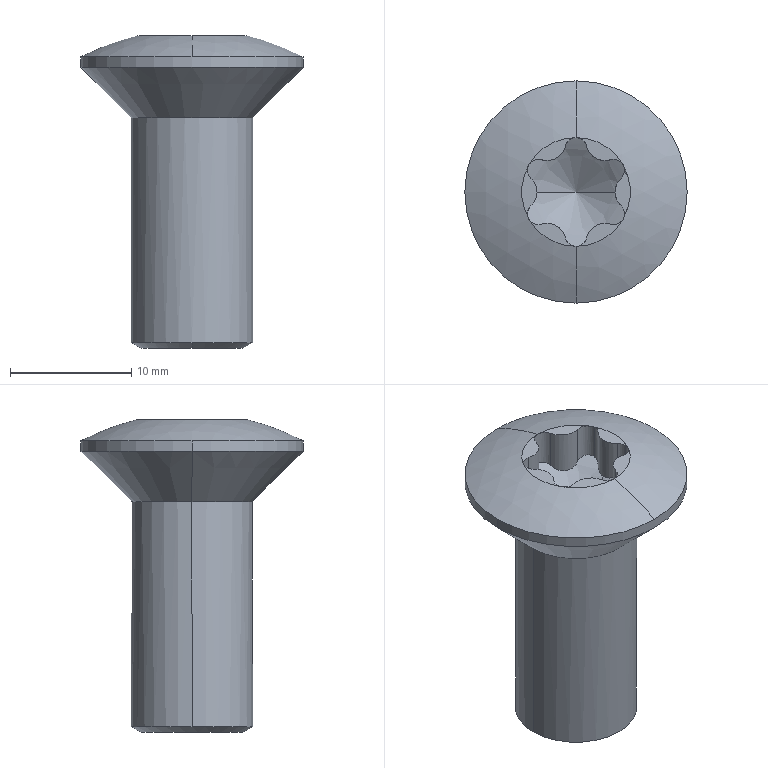Part | SolidWorks | features RevCut 2, ICE 1, LPattern 1, Revolution 1 | 1 solid | 34 faces | box 18.3 x 18.3 x 25.76 mm | volume 2486 mm3 | cylinder 19 | plane 7 | cone 6 | sphere 2 | commonest cylinder face diameters 1.79 x8 3.132 x7 10 x2 18.3 x2
STEP:
#1=CARTESIAN_POINT('',(0.,4.172,-26.28));
#2=VERTEX_POINT('',#1);
#3=CARTESIAN_POINT('',(0.,-4.172,-26.28));
#4=VERTEX_POINT('',#3);
#5=CARTESIAN_POINT('',(0.,0.,-26.28));
#6=DIRECTION('',(0.,0.,-1.));
#7=DIRECTION('',(0.,1.,0.));
#8=AXIS2_PLACEMENT_3D('',#5,#6,#7);
#9=CIRCLE('',#8,4.172);
#10=EDGE_CURVE('',#2,#4,#9,.T.);
#11=ORIENTED_EDGE('',*,*,#10,.F.);
#12=CARTESIAN_POINT('',(0.,5.,-25.802));
#13=VERTEX_POINT('',#12);
#14=CARTESIAN_POINT('',(0.,5.,-25.802));
#15=DIRECTION('',(0.,0.866,0.5));
#16=VECTOR('',#15,1000.);
#17=LINE('',#14,#16);
#18=EDGE_CURVE('',#2,#13,#17,.T.);
#19=ORIENTED_EDGE('',*,*,#18,.T.);
#20=CARTESIAN_POINT('',(5.,0.,-25.802));
#21=VERTEX_POINT('',#20);
#22=CARTESIAN_POINT('',(0.,0.,-25.802));
#23=DIRECTION('',(0.,0.,-1.));
#24=DIRECTION('',(0.,1.,0.));
#25=AXIS2_PLACEMENT_3D('',#22,#23,#24);
#26=CIRCLE('',#25,5.);
#27=EDGE_CURVE('',#13,#21,#26,.T.);
#28=ORIENTED_EDGE('',*,*,#27,.T.);
#29=CARTESIAN_POINT('',(0.,-5.,-25.802));
#30=VERTEX_POINT('',#29);
#31=CARTESIAN_POINT('',(0.,0.,-25.802));
#32=DIRECTION('',(0.,0.,-1.));
#33=DIRECTION('',(0.,1.,0.));
#34=AXIS2_PLACEMENT_3D('',#31,#32,#33);
#35=CIRCLE('',#34,5.);
#36=EDGE_CURVE('',#21,#30,#35,.T.);
#37=ORIENTED_EDGE('',*,*,#36,.T.);
#38=CARTESIAN_POINT('',(0.,-5.,-25.802));
#39=DIRECTION('',(0.,-0.866,0.5));
#40=VECTOR('',#39,1000.);
#41=LINE('',#38,#40);
#42=EDGE_CURVE('',#4,#30,#41,.T.);
#43=ORIENTED_EDGE('',*,*,#42,.F.);
#44=EDGE_LOOP('',(#11,#19,#28,#37,#43));
#45=FACE_OUTER_BOUND('',#44,.T.);
#46=CARTESIAN_POINT('',(0.,0.,-25.802));
#47=DIRECTION('',(0.,0.,1.));
#48=DIRECTION('',(0.,-1.,0.));
#49=AXIS2_PLACEMENT_3D('',#46,#47,#48);
#50=CONICAL_SURFACE('',#49,5.,1.047);
#51=ADVANCED_FACE('',(#45),#50,.T.);
#52=CARTESIAN_POINT('',(3.995,-1.79,-3.478));
#53=VERTEX_POINT('',#52);
#54=CARTESIAN_POINT('',(3.715,-1.139,-3.774));
#55=VERTEX_POINT('',#54);
#56=CARTESIAN_POINT('',(3.995,-1.79,-3.478));
#57=CARTESIAN_POINT('',(3.995,-1.663,-3.51));
#58=CARTESIAN_POINT('',(3.968,-1.538,-3.552));
#59=CARTESIAN_POINT('',(3.869,-1.316,-3.654));
#60=CARTESIAN_POINT('',(3.799,-1.219,-3.712));
#61=CARTESIAN_POINT('',(3.715,-1.139,-3.774));
#62=B_SPLINE_CURVE_WITH_KNOTS('',3,(#56,#57,#58,#59,#60,#61),.UNSPECIFIED.,.F.,.F.,(4,2,4),(0.0004714,0.0008633,0.001255),.UNSPECIFIED.);
#63=EDGE_CURVE('',#53,#55,#62,.T.);
#64=ORIENTED_EDGE('',*,*,#63,.F.);
#65=CARTESIAN_POINT('',(3.995,-1.79,-0.5204));
#66=VERTEX_POINT('',#65);
#67=CARTESIAN_POINT('',(3.995,-1.79,-500000.));
#68=DIRECTION('',(0.,0.,1.));
#69=VECTOR('',#68,1000.);
#70=LINE('',#67,#69);
#71=EDGE_CURVE('',#53,#66,#70,.T.);
#72=ORIENTED_EDGE('',*,*,#71,.T.);
#73=CARTESIAN_POINT('',(3.715,-1.139,-0.5204));
#74=VERTEX_POINT('',#73);
#75=CARTESIAN_POINT('',(3.1,-1.79,-0.5204));
#76=DIRECTION('',(0.,0.,1.));
#77=DIRECTION('',(1.,0.,0.));
#78=AXIS2_PLACEMENT_3D('',#75,#76,#77);
#79=CIRCLE('',#78,0.895);
#80=EDGE_CURVE('',#66,#74,#79,.T.);
#81=ORIENTED_EDGE('',*,*,#80,.T.);
#82=CARTESIAN_POINT('',(3.715,-1.139,-500000.));
#83=DIRECTION('',(0.,0.,1.));
#84=VECTOR('',#83,1000.);
#85=LINE('',#82,#84);
#86=EDGE_CURVE('',#55,#74,#85,.T.);
#87=ORIENTED_EDGE('',*,*,#86,.F.);
#88=EDGE_LOOP('',(#64,#72,#81,#87));
#89=FACE_OUTER_BOUND('',#88,.T.);
#90=CARTESIAN_POINT('',(3.1,-1.79,-500000.));
#91=DIRECTION('',(0.,0.,1.));
#92=DIRECTION('',(1.,0.,0.));
#93=AXIS2_PLACEMENT_3D('',#90,#91,#92);
#94=CYLINDRICAL_SURFACE('',#93,0.895);
#95=ADVANCED_FACE('',(#89),#94,.F.);
#96=CARTESIAN_POINT('',(3.995,1.79,-3.478));
#97=VERTEX_POINT('',#96);
#98=CARTESIAN_POINT('',(2.844,2.647,-3.774));
#99=VERTEX_POINT('',#98);
#100=CARTESIAN_POINT('',(3.995,1.79,-3.478));
#101=CARTESIAN_POINT('',(3.995,1.93,-3.444));
#102=CARTESIAN_POINT('',(3.962,2.073,-3.424));
#103=CARTESIAN_POINT('',(3.828,2.331,-3.417));
#104=CARTESIAN_POINT('',(3.729,2.443,-3.432));
#105=CARTESIAN_POINT('',(3.498,2.604,-3.49));
#106=CARTESIAN_POINT('',(3.365,2.655,-3.534));
#107=CARTESIAN_POINT('',(3.099,2.695,-3.642));
#108=CARTESIAN_POINT('',(2.967,2.684,-3.705));
#109=CARTESIAN_POINT('',(2.844,2.647,-3.774));
#110=B_SPLINE_CURVE_WITH_KNOTS('',3,(#100,#101,#102,#103,#104,#105,#106,#107,#108,#109),.UNSPECIFIED.,.F.,.F.,(4,2,2,2,4),(-0.0004711,-0.00003951,0.000392,0.0008236,0.001255),.UNSPECIFIED.);
#111=EDGE_CURVE('',#97,#99,#110,.T.);
#112=ORIENTED_EDGE('',*,*,#111,.F.);
#113=CARTESIAN_POINT('',(3.995,1.79,-0.5204));
#114=VERTEX_POINT('',#113);
#115=CARTESIAN_POINT('',(3.995,1.79,-500000.));
#116=DIRECTION('',(0.,0.,1.));
#117=VECTOR('',#116,1000.);
#118=LINE('',#115,#117);
#119=EDGE_CURVE('',#97,#114,#118,.T.);
#120=ORIENTED_EDGE('',*,*,#119,.T.);
#121=CARTESIAN_POINT('',(3.875,2.238,-0.5204));
#122=VERTEX_POINT('',#121);
#123=CARTESIAN_POINT('',(3.1,1.79,-0.5204));
#124=DIRECTION('',(0.,0.,1.));
#125=DIRECTION('',(1.,0.,0.));
#126=AXIS2_PLACEMENT_3D('',#123,#124,#125);
#127=CIRCLE('',#126,0.895);
#128=EDGE_CURVE('',#114,#122,#127,.T.);
#129=ORIENTED_EDGE('',*,*,#128,.T.);
#130=CARTESIAN_POINT('',(2.844,2.647,-0.5204));
#131=VERTEX_POINT('',#130);
#132=CARTESIAN_POINT('',(3.1,1.79,-0.5204));
#133=DIRECTION('',(0.,0.,1.));
#134=DIRECTION('',(1.,0.,0.));
#135=AXIS2_PLACEMENT_3D('',#132,#133,#134);
#136=CIRCLE('',#135,0.895);
#137=EDGE_CURVE('',#122,#131,#136,.T.);
#138=ORIENTED_EDGE('',*,*,#137,.T.);
#139=CARTESIAN_POINT('',(2.844,2.647,-500000.));
#140=DIRECTION('',(0.,0.,1.));
#141=VECTOR('',#140,1000.);
#142=LINE('',#139,#141);
#143=EDGE_CURVE('',#99,#131,#142,.T.);
#144=ORIENTED_EDGE('',*,*,#143,.F.);
#145=EDGE_LOOP('',(#112,#120,#129,#138,#144));
#146=FACE_OUTER_BOUND('',#145,.T.);
#147=CARTESIAN_POINT('',(3.1,1.79,-500000.));
#148=DIRECTION('',(0.,0.,1.));
#149=DIRECTION('',(1.,0.,0.));
#150=AXIS2_PLACEMENT_3D('',#147,#148,#149);
#151=CYLINDRICAL_SURFACE('',#150,0.895);
#152=ADVANCED_FACE('',(#146),#151,.F.);
#153=CARTESIAN_POINT('',(-3.715,-1.139,-3.774));
#154=VERTEX_POINT('',#153);
#155=CARTESIAN_POINT('',(-3.223,0.,-4.172));
#156=VERTEX_POINT('',#155);
#157=CARTESIAN_POINT('',(-3.715,-1.139,-3.774));
#158=CARTESIAN_POINT('',(-3.642,-1.071,-3.828));
#159=CARTESIAN_POINT('',(-3.576,-0.9953,-3.879));
#160=CARTESIAN_POINT('',(-3.457,-0.8298,-3.973));
#161=CARTESIAN_POINT('',(-3.404,-0.7384,-4.016));
#162=CARTESIAN_POINT('',(-3.274,-0.4472,-4.126));
#163=CARTESIAN_POINT('',(-3.223,-0.2243,-4.172));
#164=CARTESIAN_POINT('',(-3.223,0.,-4.172));
#165=B_SPLINE_CURVE_WITH_KNOTS('',3,(#157,#158,#159,#160,#161,#162,#163,#164),.UNSPECIFIED.,.F.,.F.,(4,2,2,4),(0.000000309,0.0003365,0.0006727,0.001345),.UNSPECIFIED.);
#166=EDGE_CURVE('',#154,#156,#165,.T.);
#167=ORIENTED_EDGE('',*,*,#166,.T.);
#168=CARTESIAN_POINT('',(-3.223,0.,-0.5204));
#169=VERTEX_POINT('',#168);
#170=CARTESIAN_POINT('',(-3.223,0.,-500000.));
#171=DIRECTION('',(0.,0.,1.));
#172=VECTOR('',#171,1000.);
#173=LINE('',#170,#172);
#174=EDGE_CURVE('',#156,#169,#173,.T.);
#175=ORIENTED_EDGE('',*,*,#174,.T.);
#176=CARTESIAN_POINT('',(-3.715,-1.139,-0.5204));
#177=VERTEX_POINT('',#176);
#178=CARTESIAN_POINT('',(-4.79,0.,-0.5204));
#179=DIRECTION('',(0.,0.,1.));
#180=DIRECTION('',(1.,0.,0.));
#181=AXIS2_PLACEMENT_3D('',#178,#179,#180);
#182=CIRCLE('',#181,1.566);
#183=EDGE_CURVE('',#177,#169,#182,.T.);
#184=ORIENTED_EDGE('',*,*,#183,.F.);
#185=CARTESIAN_POINT('',(-3.715,-1.139,-500000.));
#186=DIRECTION('',(0.,0.,1.));
#187=VECTOR('',#186,1000.);
#188=LINE('',#185,#187);
#189=EDGE_CURVE('',#154,#177,#188,.T.);
#190=ORIENTED_EDGE('',*,*,#189,.F.);
#191=EDGE_LOOP('',(#167,#175,#184,#190));
#192=FACE_OUTER_BOUND('',#191,.T.);
#193=CARTESIAN_POINT('',(-4.79,0.,-500000.));
#194=DIRECTION('',(0.,0.,1.));
#195=DIRECTION('',(1.,0.,0.));
#196=AXIS2_PLACEMENT_3D('',#193,#194,#195);
#197=CYLINDRICAL_SURFACE('',#196,1.566);
#198=ADVANCED_FACE('',(#192),#197,.T.);
#199=CARTESIAN_POINT('',(-5.,0.,-7.28));
#200=VERTEX_POINT('',#199);
#201=CARTESIAN_POINT('',(5.,0.,-7.28));
#202=VERTEX_POINT('',#201);
#203=CARTESIAN_POINT('',(0.,0.,-7.28));
#204=DIRECTION('',(0.,0.,-1.));
#205=DIRECTION('',(-1.,0.,0.));
#206=AXIS2_PLACEMENT_3D('',#203,#204,#205);
#207=CIRCLE('',#206,5.);
#208=EDGE_CURVE('',#200,#202,#207,.T.);
#209=ORIENTED_EDGE('',*,*,#208,.T.);
#210=CARTESIAN_POINT('',(5.,0.,0.));
#211=DIRECTION('',(0.,0.,-1.));
#212=VECTOR('',#211,1000.);
#213=LINE('',#210,#212);
#214=EDGE_CURVE('',#202,#21,#213,.T.);
#215=ORIENTED_EDGE('',*,*,#214,.T.);
#216=ORIENTED_EDGE('',*,*,#27,.F.);
#217=CARTESIAN_POINT('',(-5.,0.,-25.802));
#218=VERTEX_POINT('',#217);
#219=CARTESIAN_POINT('',(0.,0.,-25.802));
#220=DIRECTION('',(0.,0.,-1.));
#221=DIRECTION('',(0.,1.,0.));
#222=AXIS2_PLACEMENT_3D('',#219,#220,#221);
#223=CIRCLE('',#222,5.);
#224=EDGE_CURVE('',#218,#13,#223,.T.);
#225=ORIENTED_EDGE('',*,*,#224,.F.);
#226=CARTESIAN_POINT('',(-5.,0.,0.));
#227=DIRECTION('',(0.,0.,-1.));
#228=VECTOR('',#227,1000.);
#229=LINE('',#226,#228);
#230=EDGE_CURVE('',#200,#218,#229,.T.);
#231=ORIENTED_EDGE('',*,*,#230,.F.);
#232=EDGE_LOOP('',(#209,#215,#216,#225,#231));
#233=FACE_OUTER_BOUND('',#232,.T.);
#234=CARTESIAN_POINT('',(0.,0.,0.));
#235=DIRECTION('',(0.,0.,-1.));
#236=DIRECTION('',(-1.,0.,0.));
#237=AXIS2_PLACEMENT_3D('',#234,#235,#236);
#238=CYLINDRICAL_SURFACE('',#237,5.);
#239=ADVANCED_FACE('',(#233),#238,.T.);
#240=ORIENTED_EDGE('',*,*,#208,.F.);
#241=CARTESIAN_POINT('',(-9.15,0.,-3.13));
#242=VERTEX_POINT('',#241);
#243=CARTESIAN_POINT('',(-5.,0.,-7.28));
#244=DIRECTION('',(-0.7071,0.,0.7071));
#245=VECTOR('',#244,1000.);
#246=LINE('',#243,#245);
#247=EDGE_CURVE('',#200,#242,#246,.T.);
#248=ORIENTED_EDGE('',*,*,#247,.T.);
#249=CARTESIAN_POINT('',(9.15,0.,-3.13));
#250=VERTEX_POINT('',#249);
#251=CARTESIAN_POINT('',(0.,0.,-3.13));
#252=DIRECTION('',(0.,0.,-1.));
#253=DIRECTION('',(-1.,0.,0.));
#254=AXIS2_PLACEMENT_3D('',#251,#252,#253);
#255=CIRCLE('',#254,9.15);
#256=EDGE_CURVE('',#242,#250,#255,.T.);
#257=ORIENTED_EDGE('',*,*,#256,.T.);
#258=CARTESIAN_POINT('',(5.,0.,-7.28));
#259=DIRECTION('',(0.7071,0.,0.7071));
#260=VECTOR('',#259,1000.);
#261=LINE('',#258,#260);
#262=EDGE_CURVE('',#202,#250,#261,.T.);
#263=ORIENTED_EDGE('',*,*,#262,.F.);
#264=EDGE_LOOP('',(#240,#248,#257,#263));
#265=FACE_OUTER_BOUND('',#264,.T.);
#266=CARTESIAN_POINT('',(0.,0.,-7.28));
#267=DIRECTION('',(0.,0.,1.));
#268=DIRECTION('',(1.,0.,0.));
#269=AXIS2_PLACEMENT_3D('',#266,#267,#268);
#270=CONICAL_SURFACE('',#269,5.,0.7854);
#271=ADVANCED_FACE('',(#265),#270,.T.);
#272=CARTESIAN_POINT('',(0.,9.15,-2.28));
#273=VERTEX_POINT('',#272);
#274=CARTESIAN_POINT('',(9.15,0.,-2.28));
#275=VERTEX_POINT('',#274);
#276=CARTESIAN_POINT('',(0.,0.,-2.28));
#277=DIRECTION('',(0.,0.,-1.));
#278=DIRECTION('',(-1.,0.,0.));
#279=AXIS2_PLACEMENT_3D('',#276,#277,#278);
#280=CIRCLE('',#279,9.15);
#281=EDGE_CURVE('',#273,#275,#280,.T.);
#282=ORIENTED_EDGE('',*,*,#281,.T.);
#283=CARTESIAN_POINT('',(9.15,0.,0.));
#284=DIRECTION('',(0.,0.,-1.));
#285=VECTOR('',#284,1000.);
#286=LINE('',#283,#285);
#287=EDGE_CURVE('',#275,#250,#286,.T.);
#288=ORIENTED_EDGE('',*,*,#287,.T.);
#289=ORIENTED_EDGE('',*,*,#256,.F.);
#290=CARTESIAN_POINT('',(-9.15,0.,-2.28));
#291=VERTEX_POINT('',#290);
#292=CARTESIAN_POINT('',(-9.15,0.,0.));
#293=DIRECTION('',(0.,0.,-1.));
#294=VECTOR('',#293,1000.);
#295=LINE('',#292,#294);
#296=EDGE_CURVE('',#291,#242,#295,.T.);
#297=ORIENTED_EDGE('',*,*,#296,.F.);
#298=CARTESIAN_POINT('',(0.,0.,-2.28));
#299=DIRECTION('',(0.,0.,-1.));
#300=DIRECTION('',(-1.,0.,0.));
#301=AXIS2_PLACEMENT_3D('',#298,#299,#300);
#302=CIRCLE('',#301,9.15);
#303=EDGE_CURVE('',#291,#273,#302,.T.);
#304=ORIENTED_EDGE('',*,*,#303,.T.);
#305=EDGE_LOOP('',(#282,#288,#289,#297,#304));
#306=FACE_OUTER_BOUND('',#305,.T.);
#307=CARTESIAN_POINT('',(0.,0.,0.));
#308=DIRECTION('',(0.,0.,-1.));
#309=DIRECTION('',(-1.,0.,0.));
#310=AXIS2_PLACEMENT_3D('',#307,#308,#309);
#311=CYLINDRICAL_SURFACE('',#310,9.15);
#312=ADVANCED_FACE('',(#306),#311,.T.);
#313=CARTESIAN_POINT('',(0.,-4.475,-0.5204));
#314=VERTEX_POINT('',#313);
#315=CARTESIAN_POINT('',(3.875,-2.238,-0.5204));
#316=VERTEX_POINT('',#315);
#317=CARTESIAN_POINT('',(0.,0.,-0.5204));
#318=DIRECTION('',(0.,0.,1.));
#319=DIRECTION('',(1.,0.,0.));
#320=AXIS2_PLACEMENT_3D('',#317,#318,#319);
#321=CIRCLE('',#320,4.475);
#322=EDGE_CURVE('',#314,#316,#321,.T.);
#323=ORIENTED_EDGE('',*,*,#322,.F.);
#324=CARTESIAN_POINT('',(0.,-9.15,-2.28));
#325=VERTEX_POINT('',#324);
#326=CARTESIAN_POINT('',(0.,0.,-19.5));
#327=DIRECTION('',(1.,0.,0.));
#328=DIRECTION('',(0.,1.,0.));
#329=AXIS2_PLACEMENT_3D('',#326,#327,#328);
#330=CIRCLE('',#329,19.5);
#331=EDGE_CURVE('',#314,#325,#330,.T.);
#332=ORIENTED_EDGE('',*,*,#331,.T.);
#333=CARTESIAN_POINT('',(0.,0.,-2.28));
#334=DIRECTION('',(0.,0.,-1.));
#335=DIRECTION('',(-1.,0.,0.));
#336=AXIS2_PLACEMENT_3D('',#333,#334,#335);
#337=CIRCLE('',#336,9.15);
#338=EDGE_CURVE('',#275,#325,#337,.T.);
#339=ORIENTED_EDGE('',*,*,#338,.F.);
#340=ORIENTED_EDGE('',*,*,#281,.F.);
#341=CARTESIAN_POINT('',(0.,4.475,-0.5204));
#342=VERTEX_POINT('',#341);
#343=CARTESIAN_POINT('',(0.,0.,-19.5));
#344=DIRECTION('',(-1.,0.,0.));
#345=DIRECTION('',(0.,0.,1.));
#346=AXIS2_PLACEMENT_3D('',#343,#344,#345);
#347=CIRCLE('',#346,19.5);
#348=EDGE_CURVE('',#342,#273,#347,.T.);
#349=ORIENTED_EDGE('',*,*,#348,.F.);
#350=CARTESIAN_POINT('',(0.,0.,-0.5204));
#351=DIRECTION('',(0.,0.,1.));
#352=DIRECTION('',(1.,0.,0.));
#353=AXIS2_PLACEMENT_3D('',#350,#351,#352);
#354=CIRCLE('',#353,4.475);
#355=EDGE_CURVE('',#122,#342,#354,.T.);
#356=ORIENTED_EDGE('',*,*,#355,.F.);
#357=CARTESIAN_POINT('',(0.,0.,-0.5204));
#358=DIRECTION('',(0.,0.,1.));
#359=DIRECTION('',(1.,0.,0.));
#360=AXIS2_PLACEMENT_3D('',#357,#358,#359);
#361=CIRCLE('',#360,4.475);
#362=EDGE_CURVE('',#316,#122,#361,.T.);
#363=ORIENTED_EDGE('',*,*,#362,.F.);
#364=EDGE_LOOP('',(#323,#332,#339,#340,#349,#356,#363));
#365=FACE_OUTER_BOUND('',#364,.T.);
#366=CARTESIAN_POINT('',(0.,0.,-19.5));
#367=DIRECTION('',(1.,0.,0.));
#368=DIRECTION('',(0.,1.,0.));
#369=AXIS2_PLACEMENT_3D('',#366,#367,#368);
#370=SPHERICAL_SURFACE('',#369,19.5);
#371=ADVANCED_FACE('',(#365),#370,.T.);
#372=CARTESIAN_POINT('',(0.,0.,-6.109));
#373=VERTEX_POINT('',#372);
#374=CARTESIAN_POINT('',(3.223,0.,-4.172));
#375=VERTEX_POINT('',#374);
#376=CARTESIAN_POINT('',(0.,0.,-6.109));
#377=DIRECTION('',(0.8572,0.,0.515));
#378=VECTOR('',#377,1000.);
#379=LINE('',#376,#378);
#380=EDGE_CURVE('',#373,#375,#379,.T.);
#381=ORIENTED_EDGE('',*,*,#380,.F.);
#382=CARTESIAN_POINT('',(0.,0.,-6.109));
#383=DIRECTION('',(-0.8572,0.,0.515));
#384=VECTOR('',#383,1000.);
#385=LINE('',#382,#384);
#386=EDGE_CURVE('',#373,#156,#385,.T.);
#387=ORIENTED_EDGE('',*,*,#386,.T.);
#388=ORIENTED_EDGE('',*,*,#166,.F.);
#389=CARTESIAN_POINT('',(-2.844,-2.647,-3.774));
#390=VERTEX_POINT('',#389);
#391=CARTESIAN_POINT('',(-3.715,-1.139,-3.774));
#392=CARTESIAN_POINT('',(-3.782,-1.203,-3.724));
#393=CARTESIAN_POINT('',(-3.84,-1.277,-3.678));
#394=CARTESIAN_POINT('',(-3.932,-1.446,-3.592));
#395=CARTESIAN_POINT('',(-3.965,-1.539,-3.554));
#396=CARTESIAN_POINT('',(-4.016,-1.834,-3.458));
#397=CARTESIAN_POINT('',(-3.982,-2.052,-3.42));
#398=CARTESIAN_POINT('',(-3.823,-2.328,-3.42));
#399=CARTESIAN_POINT('',(-3.755,-2.409,-3.429));
#400=CARTESIAN_POINT('',(-3.596,-2.543,-3.463));
#401=CARTESIAN_POINT('',(-3.506,-2.594,-3.489));
#402=CARTESIAN_POINT('',(-3.224,-2.699,-3.585));
#403=CARTESIAN_POINT('',(-3.023,-2.701,-3.674));
#404=CARTESIAN_POINT('',(-2.844,-2.647,-3.774));
#405=B_SPLINE_CURVE_WITH_KNOTS('',3,(#391,#392,#393,#394,#395,#396,#397,#398,#399,#400,#401,#402,#403,#404),.UNSPECIFIED.,.F.,.F.,(4,2,2,2,2,2,4),(0.000000308,0.0003138,0.0006273,0.001254,0.001568,0.001881,0.002508),.UNSPECIFIED.);
#406=EDGE_CURVE('',#154,#390,#405,.T.);
#407=ORIENTED_EDGE('',*,*,#406,.T.);
#408=CARTESIAN_POINT('',(-0.8708,-3.787,-3.774));
#409=VERTEX_POINT('',#408);
#410=CARTESIAN_POINT('',(-0.8708,-3.787,-3.774));
#411=CARTESIAN_POINT('',(-0.8938,-3.69,-3.828));
#412=CARTESIAN_POINT('',(-0.9259,-3.595,-3.879));
#413=CARTESIAN_POINT('',(-1.01,-3.41,-3.972));
#414=CARTESIAN_POINT('',(-1.062,-3.318,-4.016));
#415=CARTESIAN_POINT('',(-1.248,-3.06,-4.126));
#416=CARTESIAN_POINT('',(-1.416,-2.905,-4.172));
#417=CARTESIAN_POINT('',(-1.706,-2.737,-4.172));
#418=CARTESIAN_POINT('',(-1.811,-2.69,-4.161));
#419=CARTESIAN_POINT('',(-2.021,-2.623,-4.12));
#420=CARTESIAN_POINT('',(-2.129,-2.601,-4.09));
#421=CARTESIAN_POINT('',(-2.446,-2.568,-3.98));
#422=CARTESIAN_POINT('',(-2.653,-2.59,-3.882));
#423=CARTESIAN_POINT('',(-2.844,-2.647,-3.774));
#424=B_SPLINE_CURVE_WITH_KNOTS('',3,(#410,#411,#412,#413,#414,#415,#416,#417,#418,#419,#420,#421,#422,#423),.UNSPECIFIED.,.F.,.F.,(4,2,2,2,2,2,4),(0.000000231,0.0003357,0.0006712,0.001342,0.001678,0.002013,0.002684),.UNSPECIFIED.);
#425=EDGE_CURVE('',#409,#390,#424,.T.);
#426=ORIENTED_EDGE('',*,*,#425,.F.);
#427=CARTESIAN_POINT('',(0.8708,-3.787,-3.774));
#428=VERTEX_POINT('',#427);
#429=CARTESIAN_POINT('',(-0.8708,-3.787,-3.774));
#430=CARTESIAN_POINT('',(-0.8493,-3.877,-3.724));
#431=CARTESIAN_POINT('',(-0.8141,-3.964,-3.678));
#432=CARTESIAN_POINT('',(-0.7139,-4.128,-3.592));
#433=CARTESIAN_POINT('',(-0.6499,-4.203,-3.554));
#434=CARTESIAN_POINT('',(-0.4201,-4.395,-3.458));
#435=CARTESIAN_POINT('',(-0.2142,-4.475,-3.42));
#436=CARTESIAN_POINT('',(0.1046,-4.475,-3.42));
#437=CARTESIAN_POINT('',(0.2086,-4.457,-3.429));
#438=CARTESIAN_POINT('',(0.4044,-4.385,-3.463));
#439=CARTESIAN_POINT('',(0.494,-4.333,-3.489));
#440=CARTESIAN_POINT('',(0.7255,-4.141,-3.585));
#441=CARTESIAN_POINT('',(0.8278,-3.968,-3.674));
#442=CARTESIAN_POINT('',(0.8708,-3.787,-3.774));
#443=B_SPLINE_CURVE_WITH_KNOTS('',3,(#429,#430,#431,#432,#433,#434,#435,#436,#437,#438,#439,#440,#441,#442),.UNSPECIFIED.,.F.,.F.,(4,2,2,2,2,2,4),(-0.001258,-0.0009439,-0.0006297,-0.00000146,0.0003127,0.0006268,0.001255),.UNSPECIFIED.);
#444=EDGE_CURVE('',#409,#428,#443,.T.);
#445=ORIENTED_EDGE('',*,*,#444,.T.);
#446=CARTESIAN_POINT('',(2.844,-2.647,-3.774));
#447=VERTEX_POINT('',#446);
#448=CARTESIAN_POINT('',(2.844,-2.647,-3.774));
#449=CARTESIAN_POINT('',(2.748,-2.619,-3.828));
#450=CARTESIAN_POINT('',(2.65,-2.599,-3.879));
#451=CARTESIAN_POINT('',(2.448,-2.579,-3.972));
#452=CARTESIAN_POINT('',(2.343,-2.579,-4.016));
#453=CARTESIAN_POINT('',(2.026,-2.611,-4.126));
#454=CARTESIAN_POINT('',(1.808,-2.679,-4.172));
#455=CARTESIAN_POINT('',(1.517,-2.846,-4.172));
#456=CARTESIAN_POINT('',(1.425,-2.913,-4.161));
#457=CARTESIAN_POINT('',(1.261,-3.062,-4.12));
#458=CARTESIAN_POINT('',(1.188,-3.144,-4.09));
#459=CARTESIAN_POINT('',(1.001,-3.403,-3.98));
#460=CARTESIAN_POINT('',(0.9169,-3.592,-3.882));
#461=CARTESIAN_POINT('',(0.8708,-3.787,-3.774));
#462=B_SPLINE_CURVE_WITH_KNOTS('',3,(#448,#449,#450,#451,#452,#453,#454,#455,#456,#457,#458,#459,#460,#461),.UNSPECIFIED.,.F.,.F.,(4,2,2,2,2,2,4),(0.000000234,0.0003357,0.0006712,0.001342,0.001678,0.002013,0.002684),.UNSPECIFIED.);
#463=EDGE_CURVE('',#447,#428,#462,.T.);
#464=ORIENTED_EDGE('',*,*,#463,.F.);
#465=CARTESIAN_POINT('',(2.844,-2.647,-3.774));
#466=CARTESIAN_POINT('',(2.967,-2.684,-3.705));
#467=CARTESIAN_POINT('',(3.099,-2.695,-3.642));
#468=CARTESIAN_POINT('',(3.297,-2.666,-3.561));
#469=CARTESIAN_POINT('',(3.363,-2.648,-3.537));
#470=CARTESIAN_POINT('',(3.491,-2.598,-3.494));
#471=CARTESIAN_POINT('',(3.554,-2.565,-3.476));
#472=CARTESIAN_POINT('',(3.727,-2.444,-3.432));
#473=CARTESIAN_POINT('',(3.827,-2.332,-3.417));
#474=CARTESIAN_POINT('',(3.961,-2.074,-3.423));
#475=CARTESIAN_POINT('',(3.995,-1.93,-3.444));
#476=CARTESIAN_POINT('',(3.995,-1.79,-3.478));
#477=B_SPLINE_CURVE_WITH_KNOTS('',3,(#465,#466,#467,#468,#469,#470,#471,#472,#473,#474,#475,#476),.UNSPECIFIED.,.F.,.F.,(4,2,2,2,2,4),(-0.001258,-0.0008256,-0.0006095,-0.0003933,0.00003904,0.0004714),.UNSPECIFIED.);
#478=EDGE_CURVE('',#447,#53,#477,.T.);
#479=ORIENTED_EDGE('',*,*,#478,.T.);
#480=ORIENTED_EDGE('',*,*,#63,.T.);
#481=CARTESIAN_POINT('',(3.223,0.,-4.172));
#482=CARTESIAN_POINT('',(3.223,-0.1117,-4.172));
#483=CARTESIAN_POINT('',(3.236,-0.2252,-4.161));
#484=CARTESIAN_POINT('',(3.283,-0.4403,-4.12));
#485=CARTESIAN_POINT('',(3.317,-0.5448,-4.09));
#486=CARTESIAN_POINT('',(3.448,-0.8352,-3.98));
#487=CARTESIAN_POINT('',(3.57,-1.002,-3.882));
#488=CARTESIAN_POINT('',(3.715,-1.139,-3.774));
#489=B_SPLINE_CURVE_WITH_KNOTS('',3,(#481,#482,#483,#484,#485,#486,#487,#488),.UNSPECIFIED.,.F.,.F.,(4,2,2,4),(0.001345,0.00168,0.002015,0.002684),.UNSPECIFIED.);
#490=EDGE_CURVE('',#375,#55,#489,.T.);
#491=ORIENTED_EDGE('',*,*,#490,.F.);
#492=EDGE_LOOP('',(#381,#387,#388,#407,#426,#445,#464,#479,#480,#491));
#493=FACE_OUTER_BOUND('',#492,.T.);
#494=CARTESIAN_POINT('',(0.,0.,993.891));
#495=DIRECTION('',(0.,0.,1.));
#496=DIRECTION('',(1.,0.,0.));
#497=AXIS2_PLACEMENT_3D('',#494,#495,#496);
#498=CONICAL_SURFACE('',#497,1664.279,1.03);
#499=ADVANCED_FACE('',(#493),#498,.F.);
#500=ORIENTED_EDGE('',*,*,#386,.F.);
#501=ORIENTED_EDGE('',*,*,#380,.T.);
#502=CARTESIAN_POINT('',(3.715,1.139,-3.774));
#503=VERTEX_POINT('',#502);
#504=CARTESIAN_POINT('',(3.715,1.139,-3.774));
#505=CARTESIAN_POINT('',(3.642,1.071,-3.828));
#506=CARTESIAN_POINT('',(3.576,0.9953,-3.879));
#507=CARTESIAN_POINT('',(3.457,0.8298,-3.973));
#508=CARTESIAN_POINT('',(3.404,0.7384,-4.016));
#509=CARTESIAN_POINT('',(3.274,0.4472,-4.126));
#510=CARTESIAN_POINT('',(3.223,0.2243,-4.172));
#511=CARTESIAN_POINT('',(3.223,0.,-4.172));
#512=B_SPLINE_CURVE_WITH_KNOTS('',3,(#504,#505,#506,#507,#508,#509,#510,#511),.UNSPECIFIED.,.F.,.F.,(4,2,2,4),(0.000000309,0.0003365,0.0006727,0.001345),.UNSPECIFIED.);
#513=EDGE_CURVE('',#503,#375,#512,.T.);
#514=ORIENTED_EDGE('',*,*,#513,.F.);
#515=CARTESIAN_POINT('',(3.715,1.139,-3.774));
#516=CARTESIAN_POINT('',(3.8,1.219,-3.711));
#517=CARTESIAN_POINT('',(3.869,1.316,-3.654));
#518=CARTESIAN_POINT('',(3.968,1.539,-3.552));
#519=CARTESIAN_POINT('',(3.995,1.662,-3.51));
#520=CARTESIAN_POINT('',(3.995,1.79,-3.478));
#521=B_SPLINE_CURVE_WITH_KNOTS('',3,(#515,#516,#517,#518,#519,#520),.UNSPECIFIED.,.F.,.F.,(4,2,4),(-0.001258,-0.0008645,-0.0004711),.UNSPECIFIED.);
#522=EDGE_CURVE('',#503,#97,#521,.T.);
#523=ORIENTED_EDGE('',*,*,#522,.T.);
#524=ORIENTED_EDGE('',*,*,#111,.T.);
#525=CARTESIAN_POINT('',(0.8708,3.787,-3.774));
#526=VERTEX_POINT('',#525);
#527=CARTESIAN_POINT('',(0.8708,3.787,-3.774));
#528=CARTESIAN_POINT('',(0.8938,3.69,-3.828));
#529=CARTESIAN_POINT('',(0.9259,3.595,-3.879));
#530=CARTESIAN_POINT('',(1.01,3.41,-3.972));
#531=CARTESIAN_POINT('',(1.062,3.318,-4.016));
#532=CARTESIAN_POINT('',(1.248,3.06,-4.126));
#533=CARTESIAN_POINT('',(1.416,2.905,-4.172));
#534=CARTESIAN_POINT('',(1.706,2.737,-4.172));
#535=CARTESIAN_POINT('',(1.811,2.69,-4.161));
#536=CARTESIAN_POINT('',(2.021,2.623,-4.12));
#537=CARTESIAN_POINT('',(2.129,2.601,-4.09));
#538=CARTESIAN_POINT('',(2.446,2.568,-3.98));
#539=CARTESIAN_POINT('',(2.653,2.59,-3.882));
#540=CARTESIAN_POINT('',(2.844,2.647,-3.774));
#541=B_SPLINE_CURVE_WITH_KNOTS('',3,(#527,#528,#529,#530,#531,#532,#533,#534,#535,#536,#537,#538,#539,#540),.UNSPECIFIED.,.F.,.F.,(4,2,2,2,2,2,4),(0.000000231,0.0003357,0.0006712,0.001342,0.001678,0.002013,0.002684),.UNSPECIFIED.);
#542=EDGE_CURVE('',#526,#99,#541,.T.);
#543=ORIENTED_EDGE('',*,*,#542,.F.);
#544=CARTESIAN_POINT('',(-0.8708,3.787,-3.774));
#545=VERTEX_POINT('',#544);
#546=CARTESIAN_POINT('',(0.8708,3.787,-3.774));
#547=CARTESIAN_POINT('',(0.8493,3.877,-3.724));
#548=CARTESIAN_POINT('',(0.8141,3.964,-3.678));
#549=CARTESIAN_POINT('',(0.7139,4.128,-3.592));
#550=CARTESIAN_POINT('',(0.6499,4.203,-3.554));
#551=CARTESIAN_POINT('',(0.4201,4.395,-3.458));
#552=CARTESIAN_POINT('',(0.2142,4.475,-3.42));
#553=CARTESIAN_POINT('',(-0.1046,4.475,-3.42));
#554=CARTESIAN_POINT('',(-0.2086,4.457,-3.429));
#555=CARTESIAN_POINT('',(-0.4044,4.385,-3.463));
#556=CARTESIAN_POINT('',(-0.494,4.333,-3.489));
#557=CARTESIAN_POINT('',(-0.7255,4.141,-3.585));
#558=CARTESIAN_POINT('',(-0.8278,3.968,-3.674));
#559=CARTESIAN_POINT('',(-0.8708,3.787,-3.774));
#560=B_SPLINE_CURVE_WITH_KNOTS('',3,(#546,#547,#548,#549,#550,#551,#552,#553,#554,#555,#556,#557,#558,#559),.UNSPECIFIED.,.F.,.F.,(4,2,2,2,2,2,4),(-0.001258,-0.0009439,-0.0006297,-0.00000146,0.0003127,0.0006268,0.001255),.UNSPECIFIED.);
#561=EDGE_CURVE('',#526,#545,#560,.T.);
#562=ORIENTED_EDGE('',*,*,#561,.T.);
#563=CARTESIAN_POINT('',(-2.844,2.647,-3.774));
#564=VERTEX_POINT('',#563);
#565=CARTESIAN_POINT('',(-2.844,2.647,-3.774));
#566=CARTESIAN_POINT('',(-2.748,2.619,-3.828));
#567=CARTESIAN_POINT('',(-2.65,2.599,-3.879));
#568=CARTESIAN_POINT('',(-2.448,2.579,-3.972));
#569=CARTESIAN_POINT('',(-2.343,2.579,-4.016));
#570=CARTESIAN_POINT('',(-2.026,2.611,-4.126));
#571=CARTESIAN_POINT('',(-1.808,2.679,-4.172));
#572=CARTESIAN_POINT('',(-1.517,2.846,-4.172));
#573=CARTESIAN_POINT('',(-1.425,2.913,-4.161));
#574=CARTESIAN_POINT('',(-1.261,3.062,-4.12));
#575=CARTESIAN_POINT('',(-1.188,3.144,-4.09));
#576=CARTESIAN_POINT('',(-1.001,3.403,-3.98));
#577=CARTESIAN_POINT('',(-0.9169,3.592,-3.882));
#578=CARTESIAN_POINT('',(-0.8708,3.787,-3.774));
#579=B_SPLINE_CURVE_WITH_KNOTS('',3,(#565,#566,#567,#568,#569,#570,#571,#572,#573,#574,#575,#576,#577,#578),.UNSPECIFIED.,.F.,.F.,(4,2,2,2,2,2,4),(0.000000234,0.0003357,0.0006712,0.001342,0.001678,0.002013,0.002684),.UNSPECIFIED.);
#580=EDGE_CURVE('',#564,#545,#579,.T.);
#581=ORIENTED_EDGE('',*,*,#580,.F.);
#582=CARTESIAN_POINT('',(-3.715,1.139,-3.774));
#583=VERTEX_POINT('',#582);
#584=CARTESIAN_POINT('',(-2.844,2.647,-3.774));
#585=CARTESIAN_POINT('',(-2.933,2.674,-3.724));
#586=CARTESIAN_POINT('',(-3.026,2.687,-3.678));
#587=CARTESIAN_POINT('',(-3.218,2.682,-3.592));
#588=CARTESIAN_POINT('',(-3.315,2.665,-3.554));
#589=CARTESIAN_POINT('',(-3.596,2.561,-3.458));
#590=CARTESIAN_POINT('',(-3.768,2.423,-3.42));
#591=CARTESIAN_POINT('',(-3.928,2.147,-3.42));
#592=CARTESIAN_POINT('',(-3.964,2.048,-3.429));
#593=CARTESIAN_POINT('',(-4.,1.842,-3.463));
#594=CARTESIAN_POINT('',(-4.,1.739,-3.489));
#595=CARTESIAN_POINT('',(-3.949,1.442,-3.585));
#596=CARTESIAN_POINT('',(-3.85,1.267,-3.674));
#597=CARTESIAN_POINT('',(-3.715,1.139,-3.774));
#598=B_SPLINE_CURVE_WITH_KNOTS('',3,(#584,#585,#586,#587,#588,#589,#590,#591,#592,#593,#594,#595,#596,#597),.UNSPECIFIED.,.F.,.F.,(4,2,2,2,2,2,4),(-0.001258,-0.0009439,-0.0006297,-0.000001429,0.0003127,0.0006269,0.001255),.UNSPECIFIED.);
#599=EDGE_CURVE('',#564,#583,#598,.T.);
#600=ORIENTED_EDGE('',*,*,#599,.T.);
#601=CARTESIAN_POINT('',(-3.223,0.,-4.172));
#602=CARTESIAN_POINT('',(-3.223,0.1117,-4.172));
#603=CARTESIAN_POINT('',(-3.236,0.2252,-4.161));
#604=CARTESIAN_POINT('',(-3.283,0.4403,-4.12));
#605=CARTESIAN_POINT('',(-3.317,0.5448,-4.09));
#606=CARTESIAN_POINT('',(-3.448,0.8352,-3.98));
#607=CARTESIAN_POINT('',(-3.57,1.002,-3.882));
#608=CARTESIAN_POINT('',(-3.715,1.139,-3.774));
#609=B_SPLINE_CURVE_WITH_KNOTS('',3,(#601,#602,#603,#604,#605,#606,#607,#608),.UNSPECIFIED.,.F.,.F.,(4,2,2,4),(0.001345,0.00168,0.002015,0.002684),.UNSPECIFIED.);
#610=EDGE_CURVE('',#156,#583,#609,.T.);
#611=ORIENTED_EDGE('',*,*,#610,.F.);
#612=EDGE_LOOP('',(#500,#501,#514,#523,#524,#543,#562,#581,#600,#611));
#613=FACE_OUTER_BOUND('',#612,.T.);
#614=CARTESIAN_POINT('',(0.,0.,993.891));
#615=DIRECTION('',(0.,0.,1.));
#616=DIRECTION('',(1.,0.,0.));
#617=AXIS2_PLACEMENT_3D('',#614,#615,#616);
#618=CONICAL_SURFACE('',#617,1664.279,1.03);
#619=ADVANCED_FACE('',(#613),#618,.F.);
#620=ORIENTED_EDGE('',*,*,#331,.F.);
#621=CARTESIAN_POINT('',(-3.875,-2.238,-0.5204));
#622=VERTEX_POINT('',#621);
#623=CARTESIAN_POINT('',(0.,0.,-0.5204));
#624=DIRECTION('',(0.,0.,1.));
#625=DIRECTION('',(-1.,0.,0.));
#626=AXIS2_PLACEMENT_3D('',#623,#624,#625);
#627=CIRCLE('',#626,4.475);
#628=EDGE_CURVE('',#622,#314,#627,.T.);
#629=ORIENTED_EDGE('',*,*,#628,.F.);
#630=CARTESIAN_POINT('',(-3.875,2.238,-0.5204));
#631=VERTEX_POINT('',#630);
#632=CARTESIAN_POINT('',(0.,0.,-0.5204));
#633=DIRECTION('',(0.,0.,1.));
#634=DIRECTION('',(1.,0.,0.));
#635=AXIS2_PLACEMENT_3D('',#632,#633,#634);
#636=CIRCLE('',#635,4.475);
#637=EDGE_CURVE('',#631,#622,#636,.T.);
#638=ORIENTED_EDGE('',*,*,#637,.F.);
#639=CARTESIAN_POINT('',(0.,0.,-0.5204));
#640=DIRECTION('',(0.,0.,1.));
#641=DIRECTION('',(1.,0.,0.));
#642=AXIS2_PLACEMENT_3D('',#639,#640,#641);
#643=CIRCLE('',#642,4.475);
#644=EDGE_CURVE('',#342,#631,#643,.T.);
#645=ORIENTED_EDGE('',*,*,#644,.F.);
#646=ORIENTED_EDGE('',*,*,#348,.T.);
#647=ORIENTED_EDGE('',*,*,#303,.F.);
#648=CARTESIAN_POINT('',(0.,0.,-2.28));
#649=DIRECTION('',(0.,0.,-1.));
#650=DIRECTION('',(-1.,0.,0.));
#651=AXIS2_PLACEMENT_3D('',#648,#649,#650);
#652=CIRCLE('',#651,9.15);
#653=EDGE_CURVE('',#325,#291,#652,.T.);
#654=ORIENTED_EDGE('',*,*,#653,.F.);
#655=EDGE_LOOP('',(#620,#629,#638,#645,#646,#647,#654));
#656=FACE_OUTER_BOUND('',#655,.T.);
#657=CARTESIAN_POINT('',(0.,0.,-19.5));
#658=DIRECTION('',(1.,0.,0.));
#659=DIRECTION('',(0.,1.,0.));
#660=AXIS2_PLACEMENT_3D('',#657,#658,#659);
#661=SPHERICAL_SURFACE('',#660,19.5);
#662=ADVANCED_FACE('',(#656),#661,.T.);
#663=ORIENTED_EDGE('',*,*,#287,.F.);
#664=ORIENTED_EDGE('',*,*,#338,.T.);
#665=ORIENTED_EDGE('',*,*,#653,.T.);
#666=ORIENTED_EDGE('',*,*,#296,.T.);
#667=CARTESIAN_POINT('',(0.,0.,-3.13));
#668=DIRECTION('',(0.,0.,-1.));
#669=DIRECTION('',(-1.,0.,0.));
#670=AXIS2_PLACEMENT_3D('',#667,#668,#669);
#671=CIRCLE('',#670,9.15);
#672=EDGE_CURVE('',#250,#242,#671,.T.);
#673=ORIENTED_EDGE('',*,*,#672,.F.);
#674=EDGE_LOOP('',(#663,#664,#665,#666,#673));
#675=FACE_OUTER_BOUND('',#674,.T.);
#676=CARTESIAN_POINT('',(0.,0.,0.));
#677=DIRECTION('',(0.,0.,-1.));
#678=DIRECTION('',(-1.,0.,0.));
#679=AXIS2_PLACEMENT_3D('',#676,#677,#678);
#680=CYLINDRICAL_SURFACE('',#679,9.15);
#681=ADVANCED_FACE('',(#675),#680,.T.);
#682=ORIENTED_EDGE('',*,*,#247,.F.);
#683=CARTESIAN_POINT('',(0.,0.,-7.28));
#684=DIRECTION('',(0.,0.,-1.));
#685=DIRECTION('',(-1.,0.,0.));
#686=AXIS2_PLACEMENT_3D('',#683,#684,#685);
#687=CIRCLE('',#686,5.);
#688=EDGE_CURVE('',#202,#200,#687,.T.);
#689=ORIENTED_EDGE('',*,*,#688,.F.);
#690=ORIENTED_EDGE('',*,*,#262,.T.);
#691=ORIENTED_EDGE('',*,*,#672,.T.);
#692=EDGE_LOOP('',(#682,#689,#690,#691));
#693=FACE_OUTER_BOUND('',#692,.T.);
#694=CARTESIAN_POINT('',(0.,0.,-7.28));
#695=DIRECTION('',(0.,0.,1.));
#696=DIRECTION('',(1.,0.,0.));
#697=AXIS2_PLACEMENT_3D('',#694,#695,#696);
#698=CONICAL_SURFACE('',#697,5.,0.7854);
#699=ADVANCED_FACE('',(#693),#698,.T.);
#700=ORIENTED_EDGE('',*,*,#214,.F.);
#701=ORIENTED_EDGE('',*,*,#688,.T.);
#702=ORIENTED_EDGE('',*,*,#230,.T.);
#703=CARTESIAN_POINT('',(0.,0.,-25.802));
#704=DIRECTION('',(0.,0.,-1.));
#705=DIRECTION('',(0.,1.,0.));
#706=AXIS2_PLACEMENT_3D('',#703,#704,#705);
#707=CIRCLE('',#706,5.);
#708=EDGE_CURVE('',#30,#218,#707,.T.);
#709=ORIENTED_EDGE('',*,*,#708,.F.);
#710=ORIENTED_EDGE('',*,*,#36,.F.);
#711=EDGE_LOOP('',(#700,#701,#702,#709,#710));
#712=FACE_OUTER_BOUND('',#711,.T.);
#713=CARTESIAN_POINT('',(0.,0.,0.));
#714=DIRECTION('',(0.,0.,-1.));
#715=DIRECTION('',(-1.,0.,0.));
#716=AXIS2_PLACEMENT_3D('',#713,#714,#715);
#717=CYLINDRICAL_SURFACE('',#716,5.);
#718=ADVANCED_FACE('',(#712),#717,.T.);
#719=CARTESIAN_POINT('',(-3.715,1.139,-0.5204));
#720=VERTEX_POINT('',#719);
#721=CARTESIAN_POINT('',(-3.1,1.79,-0.5204));
#722=DIRECTION('',(0.,0.,1.));
#723=DIRECTION('',(1.,0.,0.));
#724=AXIS2_PLACEMENT_3D('',#721,#722,#723);
#725=CIRCLE('',#724,0.895);
#726=EDGE_CURVE('',#631,#720,#725,.T.);
#727=ORIENTED_EDGE('',*,*,#726,.F.);
#728=ORIENTED_EDGE('',*,*,#637,.T.);
#729=CARTESIAN_POINT('',(-3.1,-1.79,-0.5204));
#730=DIRECTION('',(0.,0.,1.));
#731=DIRECTION('',(1.,0.,0.));
#732=AXIS2_PLACEMENT_3D('',#729,#730,#731);
#733=CIRCLE('',#732,0.895);
#734=EDGE_CURVE('',#177,#622,#733,.T.);
#735=ORIENTED_EDGE('',*,*,#734,.F.);
#736=ORIENTED_EDGE('',*,*,#183,.T.);
#737=CARTESIAN_POINT('',(-4.79,0.,-0.5204));
#738=DIRECTION('',(0.,0.,1.));
#739=DIRECTION('',(1.,0.,0.));
#740=AXIS2_PLACEMENT_3D('',#737,#738,#739);
#741=CIRCLE('',#740,1.566);
#742=EDGE_CURVE('',#169,#720,#741,.T.);
#743=ORIENTED_EDGE('',*,*,#742,.T.);
#744=EDGE_LOOP('',(#727,#728,#735,#736,#743));
#745=FACE_OUTER_BOUND('',#744,.T.);
#746=CARTESIAN_POINT('',(0.,0.,-0.5204));
#747=DIRECTION('',(0.,0.,1.));
#748=DIRECTION('',(1.,0.,0.));
#749=AXIS2_PLACEMENT_3D('',#746,#747,#748);
#750=PLANE('',#749);
#751=ADVANCED_FACE('',(#745),#750,.T.);
#752=ORIENTED_EDGE('',*,*,#599,.F.);
#753=CARTESIAN_POINT('',(-2.844,2.647,-0.5204));
#754=VERTEX_POINT('',#753);
#755=CARTESIAN_POINT('',(-2.844,2.647,-500000.));
#756=DIRECTION('',(0.,0.,1.));
#757=VECTOR('',#756,1000.);
#758=LINE('',#755,#757);
#759=EDGE_CURVE('',#564,#754,#758,.T.);
#760=ORIENTED_EDGE('',*,*,#759,.T.);
#761=CARTESIAN_POINT('',(-3.1,1.79,-0.5204));
#762=DIRECTION('',(0.,0.,1.));
#763=DIRECTION('',(1.,0.,0.));
#764=AXIS2_PLACEMENT_3D('',#761,#762,#763);
#765=CIRCLE('',#764,0.895);
#766=EDGE_CURVE('',#754,#631,#765,.T.);
#767=ORIENTED_EDGE('',*,*,#766,.T.);
#768=ORIENTED_EDGE('',*,*,#726,.T.);
#769=CARTESIAN_POINT('',(-3.715,1.139,-500000.));
#770=DIRECTION('',(0.,0.,1.));
#771=VECTOR('',#770,1000.);
#772=LINE('',#769,#771);
#773=EDGE_CURVE('',#583,#720,#772,.T.);
#774=ORIENTED_EDGE('',*,*,#773,.F.);
#775=EDGE_LOOP('',(#752,#760,#767,#768,#774));
#776=FACE_OUTER_BOUND('',#775,.T.);
#777=CARTESIAN_POINT('',(-3.1,1.79,-500000.));
#778=DIRECTION('',(0.,0.,1.));
#779=DIRECTION('',(1.,0.,0.));
#780=AXIS2_PLACEMENT_3D('',#777,#778,#779);
#781=CYLINDRICAL_SURFACE('',#780,0.895);
#782=ADVANCED_FACE('',(#776),#781,.F.);
#783=ORIENTED_EDGE('',*,*,#406,.F.);
#784=ORIENTED_EDGE('',*,*,#189,.T.);
#785=ORIENTED_EDGE('',*,*,#734,.T.);
#786=CARTESIAN_POINT('',(-2.844,-2.647,-0.5204));
#787=VERTEX_POINT('',#786);
#788=CARTESIAN_POINT('',(-3.1,-1.79,-0.5204));
#789=DIRECTION('',(0.,0.,1.));
#790=DIRECTION('',(1.,0.,0.));
#791=AXIS2_PLACEMENT_3D('',#788,#789,#790);
#792=CIRCLE('',#791,0.895);
#793=EDGE_CURVE('',#622,#787,#792,.T.);
#794=ORIENTED_EDGE('',*,*,#793,.T.);
#795=CARTESIAN_POINT('',(-2.844,-2.647,-500000.));
#796=DIRECTION('',(0.,0.,1.));
#797=VECTOR('',#796,1000.);
#798=LINE('',#795,#797);
#799=EDGE_CURVE('',#390,#787,#798,.T.);
#800=ORIENTED_EDGE('',*,*,#799,.F.);
#801=EDGE_LOOP('',(#783,#784,#785,#794,#800));
#802=FACE_OUTER_BOUND('',#801,.T.);
#803=CARTESIAN_POINT('',(-3.1,-1.79,-500000.));
#804=DIRECTION('',(0.,0.,1.));
#805=DIRECTION('',(1.,0.,0.));
#806=AXIS2_PLACEMENT_3D('',#803,#804,#805);
#807=CYLINDRICAL_SURFACE('',#806,0.895);
#808=ADVANCED_FACE('',(#802),#807,.F.);
#809=ORIENTED_EDGE('',*,*,#174,.F.);
#810=ORIENTED_EDGE('',*,*,#610,.T.);
#811=ORIENTED_EDGE('',*,*,#773,.T.);
#812=ORIENTED_EDGE('',*,*,#742,.F.);
#813=EDGE_LOOP('',(#809,#810,#811,#812));
#814=FACE_OUTER_BOUND('',#813,.T.);
#815=CARTESIAN_POINT('',(-4.79,0.,-500000.));
#816=DIRECTION('',(0.,0.,1.));
#817=DIRECTION('',(1.,0.,0.));
#818=AXIS2_PLACEMENT_3D('',#815,#816,#817);
#819=CYLINDRICAL_SURFACE('',#818,1.566);
#820=ADVANCED_FACE('',(#814),#819,.T.);
#821=CARTESIAN_POINT('',(-0.8708,3.787,-0.5204));
#822=VERTEX_POINT('',#821);
#823=CARTESIAN_POINT('',(0.,3.58,-0.5204));
#824=DIRECTION('',(0.,0.,1.));
#825=DIRECTION('',(1.,0.,0.));
#826=AXIS2_PLACEMENT_3D('',#823,#824,#825);
#827=CIRCLE('',#826,0.895);
#828=EDGE_CURVE('',#342,#822,#827,.T.);
#829=ORIENTED_EDGE('',*,*,#828,.F.);
#830=ORIENTED_EDGE('',*,*,#644,.T.);
#831=ORIENTED_EDGE('',*,*,#766,.F.);
#832=CARTESIAN_POINT('',(-2.395,4.148,-0.5204));
#833=DIRECTION('',(0.,0.,1.));
#834=DIRECTION('',(1.,0.,0.));
#835=AXIS2_PLACEMENT_3D('',#832,#833,#834);
#836=CIRCLE('',#835,1.566);
#837=EDGE_CURVE('',#754,#822,#836,.T.);
#838=ORIENTED_EDGE('',*,*,#837,.T.);
#839=EDGE_LOOP('',(#829,#830,#831,#838));
#840=FACE_OUTER_BOUND('',#839,.T.);
#841=CARTESIAN_POINT('',(0.,0.,-0.5204));
#842=DIRECTION('',(0.,0.,1.));
#843=DIRECTION('',(1.,0.,0.));
#844=AXIS2_PLACEMENT_3D('',#841,#842,#843);
#845=PLANE('',#844);
#846=ADVANCED_FACE('',(#840),#845,.T.);
#847=ORIENTED_EDGE('',*,*,#561,.F.);
#848=CARTESIAN_POINT('',(0.8708,3.787,-0.5204));
#849=VERTEX_POINT('',#848);
#850=CARTESIAN_POINT('',(0.8708,3.787,-500000.));
#851=DIRECTION('',(0.,0.,1.));
#852=VECTOR('',#851,1000.);
#853=LINE('',#850,#852);
#854=EDGE_CURVE('',#526,#849,#853,.T.);
#855=ORIENTED_EDGE('',*,*,#854,.T.);
#856=CARTESIAN_POINT('',(0.,3.58,-0.5204));
#857=DIRECTION('',(0.,0.,1.));
#858=DIRECTION('',(1.,0.,0.));
#859=AXIS2_PLACEMENT_3D('',#856,#857,#858);
#860=CIRCLE('',#859,0.895);
#861=EDGE_CURVE('',#849,#342,#860,.T.);
#862=ORIENTED_EDGE('',*,*,#861,.T.);
#863=ORIENTED_EDGE('',*,*,#828,.T.);
#864=CARTESIAN_POINT('',(-0.8708,3.787,-500000.));
#865=DIRECTION('',(0.,0.,1.));
#866=VECTOR('',#865,1000.);
#867=LINE('',#864,#866);
#868=EDGE_CURVE('',#545,#822,#867,.T.);
#869=ORIENTED_EDGE('',*,*,#868,.F.);
#870=EDGE_LOOP('',(#847,#855,#862,#863,#869));
#871=FACE_OUTER_BOUND('',#870,.T.);
#872=CARTESIAN_POINT('',(0.,3.58,-500000.));
#873=DIRECTION('',(0.,0.,1.));
#874=DIRECTION('',(1.,0.,0.));
#875=AXIS2_PLACEMENT_3D('',#872,#873,#874);
#876=CYLINDRICAL_SURFACE('',#875,0.895);
#877=ADVANCED_FACE('',(#871),#876,.F.);
#878=ORIENTED_EDGE('',*,*,#759,.F.);
#879=ORIENTED_EDGE('',*,*,#580,.T.);
#880=ORIENTED_EDGE('',*,*,#868,.T.);
#881=ORIENTED_EDGE('',*,*,#837,.F.);
#882=EDGE_LOOP('',(#878,#879,#880,#881));
#883=FACE_OUTER_BOUND('',#882,.T.);
#884=CARTESIAN_POINT('',(-2.395,4.148,-500000.));
#885=DIRECTION('',(0.,0.,1.));
#886=DIRECTION('',(1.,0.,0.));
#887=AXIS2_PLACEMENT_3D('',#884,#885,#886);
#888=CYLINDRICAL_SURFACE('',#887,1.566);
#889=ADVANCED_FACE('',(#883),#888,.T.);
#890=ORIENTED_EDGE('',*,*,#137,.F.);
#891=ORIENTED_EDGE('',*,*,#355,.T.);
#892=ORIENTED_EDGE('',*,*,#861,.F.);
#893=CARTESIAN_POINT('',(2.395,4.148,-0.5204));
#894=DIRECTION('',(0.,0.,1.));
#895=DIRECTION('',(1.,0.,0.));
#896=AXIS2_PLACEMENT_3D('',#893,#894,#895);
#897=CIRCLE('',#896,1.566);
#898=EDGE_CURVE('',#849,#131,#897,.T.);
#899=ORIENTED_EDGE('',*,*,#898,.T.);
#900=EDGE_LOOP('',(#890,#891,#892,#899));
#901=FACE_OUTER_BOUND('',#900,.T.);
#902=CARTESIAN_POINT('',(0.,0.,-0.5204));
#903=DIRECTION('',(0.,0.,1.));
#904=DIRECTION('',(1.,0.,0.));
#905=AXIS2_PLACEMENT_3D('',#902,#903,#904);
#906=PLANE('',#905);
#907=ADVANCED_FACE('',(#901),#906,.T.);
#908=ORIENTED_EDGE('',*,*,#119,.F.);
#909=ORIENTED_EDGE('',*,*,#522,.F.);
#910=CARTESIAN_POINT('',(3.715,1.139,-0.5204));
#911=VERTEX_POINT('',#910);
#912=CARTESIAN_POINT('',(3.715,1.139,-500000.));
#913=DIRECTION('',(0.,0.,1.));
#914=VECTOR('',#913,1000.);
#915=LINE('',#912,#914);
#916=EDGE_CURVE('',#503,#911,#915,.T.);
#917=ORIENTED_EDGE('',*,*,#916,.T.);
#918=CARTESIAN_POINT('',(3.1,1.79,-0.5204));
#919=DIRECTION('',(0.,0.,1.));
#920=DIRECTION('',(1.,0.,0.));
#921=AXIS2_PLACEMENT_3D('',#918,#919,#920);
#922=CIRCLE('',#921,0.895);
#923=EDGE_CURVE('',#911,#114,#922,.T.);
#924=ORIENTED_EDGE('',*,*,#923,.T.);
#925=EDGE_LOOP('',(#908,#909,#917,#924));
#926=FACE_OUTER_BOUND('',#925,.T.);
#927=CARTESIAN_POINT('',(3.1,1.79,-500000.));
#928=DIRECTION('',(0.,0.,1.));
#929=DIRECTION('',(1.,0.,0.));
#930=AXIS2_PLACEMENT_3D('',#927,#928,#929);
#931=CYLINDRICAL_SURFACE('',#930,0.895);
#932=ADVANCED_FACE('',(#926),#931,.F.);
#933=ORIENTED_EDGE('',*,*,#854,.F.);
#934=ORIENTED_EDGE('',*,*,#542,.T.);
#935=ORIENTED_EDGE('',*,*,#143,.T.);
#936=ORIENTED_EDGE('',*,*,#898,.F.);
#937=EDGE_LOOP('',(#933,#934,#935,#936));
#938=FACE_OUTER_BOUND('',#937,.T.);
#939=CARTESIAN_POINT('',(2.395,4.148,-500000.));
#940=DIRECTION('',(0.,0.,1.));
#941=DIRECTION('',(1.,0.,0.));
#942=AXIS2_PLACEMENT_3D('',#939,#940,#941);
#943=CYLINDRICAL_SURFACE('',#942,1.566);
#944=ADVANCED_FACE('',(#938),#943,.T.);
#945=CARTESIAN_POINT('',(3.1,-1.79,-0.5204));
#946=DIRECTION('',(0.,0.,1.));
#947=DIRECTION('',(1.,0.,0.));
#948=AXIS2_PLACEMENT_3D('',#945,#946,#947);
#949=CIRCLE('',#948,0.895);
#950=EDGE_CURVE('',#316,#66,#949,.T.);
#951=ORIENTED_EDGE('',*,*,#950,.F.);
#952=ORIENTED_EDGE('',*,*,#362,.T.);
#953=ORIENTED_EDGE('',*,*,#128,.F.);
#954=ORIENTED_EDGE('',*,*,#923,.F.);
#955=CARTESIAN_POINT('',(4.79,0.,-0.5204));
#956=DIRECTION('',(0.,0.,1.));
#957=DIRECTION('',(1.,0.,0.));
#958=AXIS2_PLACEMENT_3D('',#955,#956,#957);
#959=CIRCLE('',#958,1.566);
#960=EDGE_CURVE('',#911,#74,#959,.T.);
#961=ORIENTED_EDGE('',*,*,#960,.T.);
#962=ORIENTED_EDGE('',*,*,#80,.F.);
#963=EDGE_LOOP('',(#951,#952,#953,#954,#961,#962));
#964=FACE_OUTER_BOUND('',#963,.T.);
#965=CARTESIAN_POINT('',(0.,0.,-0.5204));
#966=DIRECTION('',(0.,0.,1.));
#967=DIRECTION('',(1.,0.,0.));
#968=AXIS2_PLACEMENT_3D('',#965,#966,#967);
#969=PLANE('',#968);
#970=ADVANCED_FACE('',(#964),#969,.T.);
#971=ORIENTED_EDGE('',*,*,#71,.F.);
#972=ORIENTED_EDGE('',*,*,#478,.F.);
#973=CARTESIAN_POINT('',(2.844,-2.647,-0.5204));
#974=VERTEX_POINT('',#973);
#975=CARTESIAN_POINT('',(2.844,-2.647,-500000.));
#976=DIRECTION('',(0.,0.,1.));
#977=VECTOR('',#976,1000.);
#978=LINE('',#975,#977);
#979=EDGE_CURVE('',#447,#974,#978,.T.);
#980=ORIENTED_EDGE('',*,*,#979,.T.);
#981=CARTESIAN_POINT('',(3.1,-1.79,-0.5204));
#982=DIRECTION('',(0.,0.,1.));
#983=DIRECTION('',(1.,0.,0.));
#984=AXIS2_PLACEMENT_3D('',#981,#982,#983);
#985=CIRCLE('',#984,0.895);
#986=EDGE_CURVE('',#974,#316,#985,.T.);
#987=ORIENTED_EDGE('',*,*,#986,.T.);
#988=ORIENTED_EDGE('',*,*,#950,.T.);
#989=EDGE_LOOP('',(#971,#972,#980,#987,#988));
#990=FACE_OUTER_BOUND('',#989,.T.);
#991=CARTESIAN_POINT('',(3.1,-1.79,-500000.));
#992=DIRECTION('',(0.,0.,1.));
#993=DIRECTION('',(1.,0.,0.));
#994=AXIS2_PLACEMENT_3D('',#991,#992,#993);
#995=CYLINDRICAL_SURFACE('',#994,0.895);
#996=ADVANCED_FACE('',(#990),#995,.F.);
#997=ORIENTED_EDGE('',*,*,#916,.F.);
#998=ORIENTED_EDGE('',*,*,#513,.T.);
#999=ORIENTED_EDGE('',*,*,#490,.T.);
#1000=ORIENTED_EDGE('',*,*,#86,.T.);
#1001=ORIENTED_EDGE('',*,*,#960,.F.);
#1002=EDGE_LOOP('',(#997,#998,#999,#1000,#1001));
#1003=FACE_OUTER_BOUND('',#1002,.T.);
#1004=CARTESIAN_POINT('',(4.79,0.,-500000.));
#1005=DIRECTION('',(0.,0.,1.));
#1006=DIRECTION('',(1.,0.,0.));
#1007=AXIS2_PLACEMENT_3D('',#1004,#1005,#1006);
#1008=CYLINDRICAL_SURFACE('',#1007,1.566);
#1009=ADVANCED_FACE('',(#1003),#1008,.T.);
#1010=CARTESIAN_POINT('',(0.8708,-3.787,-0.5204));
#1011=VERTEX_POINT('',#1010);
#1012=CARTESIAN_POINT('',(0.,-3.58,-0.5204));
#1013=DIRECTION('',(0.,0.,1.));
#1014=DIRECTION('',(1.,0.,0.));
#1015=AXIS2_PLACEMENT_3D('',#1012,#1013,#1014);
#1016=CIRCLE('',#1015,0.895);
#1017=EDGE_CURVE('',#314,#1011,#1016,.T.);
#1018=ORIENTED_EDGE('',*,*,#1017,.F.);
#1019=ORIENTED_EDGE('',*,*,#322,.T.);
#1020=ORIENTED_EDGE('',*,*,#986,.F.);
#1021=CARTESIAN_POINT('',(2.395,-4.148,-0.5204));
#1022=DIRECTION('',(0.,0.,1.));
#1023=DIRECTION('',(1.,0.,0.));
#1024=AXIS2_PLACEMENT_3D('',#1021,#1022,#1023);
#1025=CIRCLE('',#1024,1.566);
#1026=EDGE_CURVE('',#974,#1011,#1025,.T.);
#1027=ORIENTED_EDGE('',*,*,#1026,.T.);
#1028=EDGE_LOOP('',(#1018,#1019,#1020,#1027));
#1029=FACE_OUTER_BOUND('',#1028,.T.);
#1030=CARTESIAN_POINT('',(0.,0.,-0.5204));
#1031=DIRECTION('',(0.,0.,1.));
#1032=DIRECTION('',(1.,0.,0.));
#1033=AXIS2_PLACEMENT_3D('',#1030,#1031,#1032);
#1034=PLANE('',#1033);
#1035=ADVANCED_FACE('',(#1029),#1034,.T.);
#1036=ORIENTED_EDGE('',*,*,#444,.F.);
#1037=CARTESIAN_POINT('',(-0.8708,-3.787,-0.5204));
#1038=VERTEX_POINT('',#1037);
#1039=CARTESIAN_POINT('',(-0.8708,-3.787,-500000.));
#1040=DIRECTION('',(0.,0.,1.));
#1041=VECTOR('',#1040,1000.);
#1042=LINE('',#1039,#1041);
#1043=EDGE_CURVE('',#409,#1038,#1042,.T.);
#1044=ORIENTED_EDGE('',*,*,#1043,.T.);
#1045=CARTESIAN_POINT('',(0.,-3.58,-0.5204));
#1046=DIRECTION('',(0.,0.,1.));
#1047=DIRECTION('',(1.,0.,0.));
#1048=AXIS2_PLACEMENT_3D('',#1045,#1046,#1047);
#1049=CIRCLE('',#1048,0.895);
#1050=EDGE_CURVE('',#1038,#314,#1049,.T.);
#1051=ORIENTED_EDGE('',*,*,#1050,.T.);
#1052=ORIENTED_EDGE('',*,*,#1017,.T.);
#1053=CARTESIAN_POINT('',(0.8708,-3.787,-500000.));
#1054=DIRECTION('',(0.,0.,1.));
#1055=VECTOR('',#1054,1000.);
#1056=LINE('',#1053,#1055);
#1057=EDGE_CURVE('',#428,#1011,#1056,.T.);
#1058=ORIENTED_EDGE('',*,*,#1057,.F.);
#1059=EDGE_LOOP('',(#1036,#1044,#1051,#1052,#1058));
#1060=FACE_OUTER_BOUND('',#1059,.T.);
#1061=CARTESIAN_POINT('',(0.,-3.58,-500000.));
#1062=DIRECTION('',(0.,0.,1.));
#1063=DIRECTION('',(1.,0.,0.));
#1064=AXIS2_PLACEMENT_3D('',#1061,#1062,#1063);
#1065=CYLINDRICAL_SURFACE('',#1064,0.895);
#1066=ADVANCED_FACE('',(#1060),#1065,.F.);
#1067=ORIENTED_EDGE('',*,*,#979,.F.);
#1068=ORIENTED_EDGE('',*,*,#463,.T.);
#1069=ORIENTED_EDGE('',*,*,#1057,.T.);
#1070=ORIENTED_EDGE('',*,*,#1026,.F.);
#1071=EDGE_LOOP('',(#1067,#1068,#1069,#1070));
#1072=FACE_OUTER_BOUND('',#1071,.T.);
#1073=CARTESIAN_POINT('',(2.395,-4.148,-500000.));
#1074=DIRECTION('',(0.,0.,1.));
#1075=DIRECTION('',(1.,0.,0.));
#1076=AXIS2_PLACEMENT_3D('',#1073,#1074,#1075);
#1077=CYLINDRICAL_SURFACE('',#1076,1.566);
#1078=ADVANCED_FACE('',(#1072),#1077,.T.);
#1079=ORIENTED_EDGE('',*,*,#793,.F.);
#1080=ORIENTED_EDGE('',*,*,#628,.T.);
#1081=ORIENTED_EDGE('',*,*,#1050,.F.);
#1082=CARTESIAN_POINT('',(-2.395,-4.148,-0.5204));
#1083=DIRECTION('',(0.,0.,1.));
#1084=DIRECTION('',(1.,0.,0.));
#1085=AXIS2_PLACEMENT_3D('',#1082,#1083,#1084);
#1086=CIRCLE('',#1085,1.566);
#1087=EDGE_CURVE('',#1038,#787,#1086,.T.);
#1088=ORIENTED_EDGE('',*,*,#1087,.T.);
#1089=EDGE_LOOP('',(#1079,#1080,#1081,#1088));
#1090=FACE_OUTER_BOUND('',#1089,.T.);
#1091=CARTESIAN_POINT('',(0.,0.,-0.5204));
#1092=DIRECTION('',(0.,0.,1.));
#1093=DIRECTION('',(1.,0.,0.));
#1094=AXIS2_PLACEMENT_3D('',#1091,#1092,#1093);
#1095=PLANE('',#1094);
#1096=ADVANCED_FACE('',(#1090),#1095,.T.);
#1097=ORIENTED_EDGE('',*,*,#1043,.F.);
#1098=ORIENTED_EDGE('',*,*,#425,.T.);
#1099=ORIENTED_EDGE('',*,*,#799,.T.);
#1100=ORIENTED_EDGE('',*,*,#1087,.F.);
#1101=EDGE_LOOP('',(#1097,#1098,#1099,#1100));
#1102=FACE_OUTER_BOUND('',#1101,.T.);
#1103=CARTESIAN_POINT('',(-2.395,-4.148,-500000.));
#1104=DIRECTION('',(0.,0.,1.));
#1105=DIRECTION('',(1.,0.,0.));
#1106=AXIS2_PLACEMENT_3D('',#1103,#1104,#1105);
#1107=CYLINDRICAL_SURFACE('',#1106,1.566);
#1108=ADVANCED_FACE('',(#1102),#1107,.T.);
#1109=ORIENTED_EDGE('',*,*,#18,.F.);
#1110=CARTESIAN_POINT('',(0.,0.,-26.28));
#1111=DIRECTION('',(0.,0.,-1.));
#1112=DIRECTION('',(0.,1.,0.));
#1113=AXIS2_PLACEMENT_3D('',#1110,#1111,#1112);
#1114=CIRCLE('',#1113,4.172);
#1115=EDGE_CURVE('',#4,#2,#1114,.T.);
#1116=ORIENTED_EDGE('',*,*,#1115,.F.);
#1117=ORIENTED_EDGE('',*,*,#42,.T.);
#1118=ORIENTED_EDGE('',*,*,#708,.T.);
#1119=ORIENTED_EDGE('',*,*,#224,.T.);
#1120=EDGE_LOOP('',(#1109,#1116,#1117,#1118,#1119));
#1121=FACE_OUTER_BOUND('',#1120,.T.);
#1122=CARTESIAN_POINT('',(0.,0.,-25.802));
#1123=DIRECTION('',(0.,0.,1.));
#1124=DIRECTION('',(0.,-1.,0.));
#1125=AXIS2_PLACEMENT_3D('',#1122,#1123,#1124);
#1126=CONICAL_SURFACE('',#1125,5.,1.047);
#1127=ADVANCED_FACE('',(#1121),#1126,.T.);
#1128=ORIENTED_EDGE('',*,*,#1115,.T.);
#1129=ORIENTED_EDGE('',*,*,#10,.T.);
#1130=EDGE_LOOP('',(#1128,#1129));
#1131=FACE_OUTER_BOUND('',#1130,.T.);
#1132=CARTESIAN_POINT('',(0.,5.,-26.28));
#1133=DIRECTION('',(0.,0.,-1.));
#1134=DIRECTION('',(-1.,0.,0.));
#1135=AXIS2_PLACEMENT_3D('',#1132,#1133,#1134);
#1136=PLANE('',#1135);
#1137=ADVANCED_FACE('',(#1131),#1136,.T.);
#1138=CLOSED_SHELL('',(#51,#95,#152,#198,#239,#271,#312,#371,#499,#619,#662,#681,#699,#718,#751,#782,#808,#820,#846,#877,#889,#907,#932,#944,#970,#996,#1009,#1035,#1066,#1078,#1096,#1108,#1127,#1137));
#1139=MANIFOLD_SOLID_BREP('',#1138);
#1140=CARTESIAN_POINT('',(0.,0.,0.));
#1141=DIRECTION('',(0.,0.,1.));
#1142=DIRECTION('',(1.,0.,0.));
#1143=AXIS2_PLACEMENT_3D('',#1140,#1141,#1142);
#1144=(LENGTH_UNIT()NAMED_UNIT(*)SI_UNIT(.MILLI.,.METRE.));
#1145=UNCERTAINTY_MEASURE_WITH_UNIT(LENGTH_MEASURE(0.00001),#1144,'','');
#1146=(NAMED_UNIT(*)PLANE_ANGLE_UNIT()SI_UNIT($,.RADIAN.));
#1147=(NAMED_UNIT(*)SI_UNIT($,.STERADIAN.)SOLID_ANGLE_UNIT());
#1148=(GEOMETRIC_REPRESENTATION_CONTEXT(3)GLOBAL_UNCERTAINTY_ASSIGNED_CONTEXT((#1145))GLOBAL_UNIT_ASSIGNED_CONTEXT((#1144,#1146,#1147))REPRESENTATION_CONTEXT('',''));
#1149=ADVANCED_BREP_SHAPE_REPRESENTATION('',(#1139,#1143),#1148);